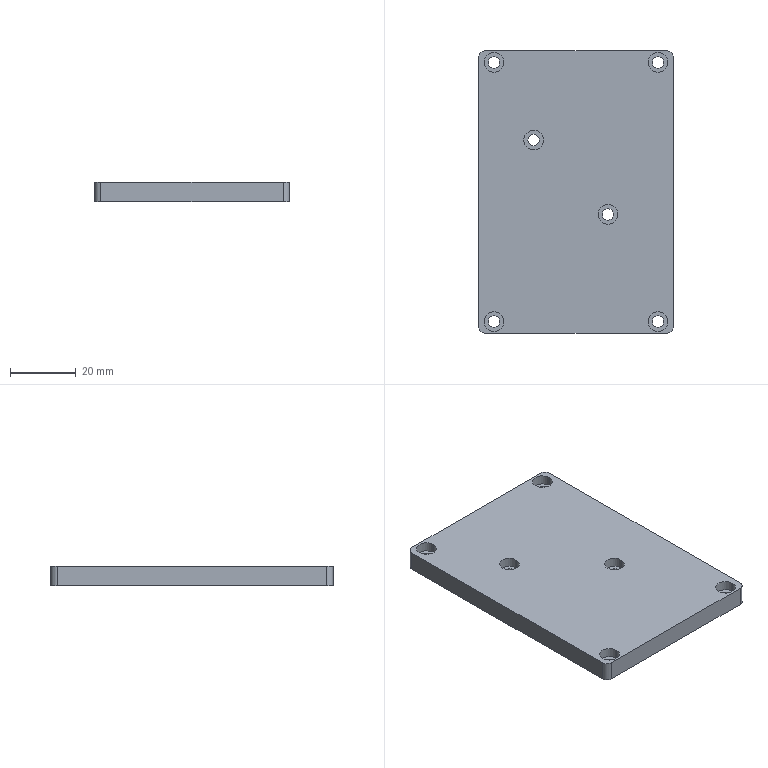Part | SolidWorks | features ICE 2, Extrusion 1, Fillet 1 | 1 solid | 40 faces | box 59.5 x 86 x 6 mm | volume 29999 mm3 | cylinder 28 | plane 12 | commonest cylinder face diameters 3.5 x12 6 x12 4 x4
STEP:
#1=CARTESIAN_POINT('',(22.,-39.5,3.));
#2=VERTEX_POINT('',#1);
#3=CARTESIAN_POINT('',(28.,-39.5,3.));
#4=VERTEX_POINT('',#3);
#5=CARTESIAN_POINT('',(25.,-39.5,3.));
#6=DIRECTION('',(0.,0.,1.));
#7=DIRECTION('',(1.,0.,0.));
#8=AXIS2_PLACEMENT_3D('',#5,#6,#7);
#9=CIRCLE('',#8,3.);
#10=EDGE_CURVE('',#2,#4,#9,.T.);
#11=ORIENTED_EDGE('',*,*,#10,.F.);
#12=CARTESIAN_POINT('',(22.,-39.5,6.));
#13=VERTEX_POINT('',#12);
#14=CARTESIAN_POINT('',(22.,-39.5,3.));
#15=DIRECTION('',(0.,0.,1.));
#16=VECTOR('',#15,1000.);
#17=LINE('',#14,#16);
#18=EDGE_CURVE('',#2,#13,#17,.T.);
#19=ORIENTED_EDGE('',*,*,#18,.T.);
#20=CARTESIAN_POINT('',(28.,-39.5,6.));
#21=VERTEX_POINT('',#20);
#22=CARTESIAN_POINT('',(25.,-39.5,6.));
#23=DIRECTION('',(0.,0.,1.));
#24=DIRECTION('',(1.,0.,0.));
#25=AXIS2_PLACEMENT_3D('',#22,#23,#24);
#26=CIRCLE('',#25,3.);
#27=EDGE_CURVE('',#13,#21,#26,.T.);
#28=ORIENTED_EDGE('',*,*,#27,.T.);
#29=CARTESIAN_POINT('',(28.,-39.5,3.));
#30=DIRECTION('',(0.,0.,1.));
#31=VECTOR('',#30,1000.);
#32=LINE('',#29,#31);
#33=EDGE_CURVE('',#4,#21,#32,.T.);
#34=ORIENTED_EDGE('',*,*,#33,.F.);
#35=EDGE_LOOP('',(#11,#19,#28,#34));
#36=FACE_OUTER_BOUND('',#35,.T.);
#37=CARTESIAN_POINT('',(25.,-39.5,3.));
#38=DIRECTION('',(0.,0.,1.));
#39=DIRECTION('',(1.,0.,0.));
#40=AXIS2_PLACEMENT_3D('',#37,#38,#39);
#41=CYLINDRICAL_SURFACE('',#40,3.);
#42=ADVANCED_FACE('',(#36),#41,.F.);
#43=CARTESIAN_POINT('',(-28.,-39.5,3.));
#44=VERTEX_POINT('',#43);
#45=CARTESIAN_POINT('',(-22.,-39.5,3.));
#46=VERTEX_POINT('',#45);
#47=CARTESIAN_POINT('',(-25.,-39.5,3.));
#48=DIRECTION('',(0.,0.,1.));
#49=DIRECTION('',(1.,0.,0.));
#50=AXIS2_PLACEMENT_3D('',#47,#48,#49);
#51=CIRCLE('',#50,3.);
#52=EDGE_CURVE('',#44,#46,#51,.T.);
#53=ORIENTED_EDGE('',*,*,#52,.F.);
#54=CARTESIAN_POINT('',(-28.,-39.5,6.));
#55=VERTEX_POINT('',#54);
#56=CARTESIAN_POINT('',(-28.,-39.5,3.));
#57=DIRECTION('',(0.,0.,1.));
#58=VECTOR('',#57,1000.);
#59=LINE('',#56,#58);
#60=EDGE_CURVE('',#44,#55,#59,.T.);
#61=ORIENTED_EDGE('',*,*,#60,.T.);
#62=CARTESIAN_POINT('',(-22.,-39.5,6.));
#63=VERTEX_POINT('',#62);
#64=CARTESIAN_POINT('',(-25.,-39.5,6.));
#65=DIRECTION('',(0.,0.,1.));
#66=DIRECTION('',(1.,0.,0.));
#67=AXIS2_PLACEMENT_3D('',#64,#65,#66);
#68=CIRCLE('',#67,3.);
#69=EDGE_CURVE('',#55,#63,#68,.T.);
#70=ORIENTED_EDGE('',*,*,#69,.T.);
#71=CARTESIAN_POINT('',(-22.,-39.5,3.));
#72=DIRECTION('',(0.,0.,1.));
#73=VECTOR('',#72,1000.);
#74=LINE('',#71,#73);
#75=EDGE_CURVE('',#46,#63,#74,.T.);
#76=ORIENTED_EDGE('',*,*,#75,.F.);
#77=EDGE_LOOP('',(#53,#61,#70,#76));
#78=FACE_OUTER_BOUND('',#77,.T.);
#79=CARTESIAN_POINT('',(-25.,-39.5,3.));
#80=DIRECTION('',(0.,0.,1.));
#81=DIRECTION('',(1.,0.,0.));
#82=AXIS2_PLACEMENT_3D('',#79,#80,#81);
#83=CYLINDRICAL_SURFACE('',#82,3.);
#84=ADVANCED_FACE('',(#78),#83,.F.);
#85=CARTESIAN_POINT('',(6.727,-6.827,3.));
#86=VERTEX_POINT('',#85);
#87=CARTESIAN_POINT('',(12.727,-6.827,3.));
#88=VERTEX_POINT('',#87);
#89=CARTESIAN_POINT('',(9.727,-6.827,3.));
#90=DIRECTION('',(0.,0.,1.));
#91=DIRECTION('',(1.,0.,0.));
#92=AXIS2_PLACEMENT_3D('',#89,#90,#91);
#93=CIRCLE('',#92,3.);
#94=EDGE_CURVE('',#86,#88,#93,.T.);
#95=ORIENTED_EDGE('',*,*,#94,.F.);
#96=CARTESIAN_POINT('',(6.727,-6.827,6.));
#97=VERTEX_POINT('',#96);
#98=CARTESIAN_POINT('',(6.727,-6.827,3.));
#99=DIRECTION('',(0.,0.,1.));
#100=VECTOR('',#99,1000.);
#101=LINE('',#98,#100);
#102=EDGE_CURVE('',#86,#97,#101,.T.);
#103=ORIENTED_EDGE('',*,*,#102,.T.);
#104=CARTESIAN_POINT('',(12.727,-6.827,6.));
#105=VERTEX_POINT('',#104);
#106=CARTESIAN_POINT('',(9.727,-6.827,6.));
#107=DIRECTION('',(0.,0.,1.));
#108=DIRECTION('',(1.,0.,0.));
#109=AXIS2_PLACEMENT_3D('',#106,#107,#108);
#110=CIRCLE('',#109,3.);
#111=EDGE_CURVE('',#97,#105,#110,.T.);
#112=ORIENTED_EDGE('',*,*,#111,.T.);
#113=CARTESIAN_POINT('',(12.727,-6.827,3.));
#114=DIRECTION('',(0.,0.,1.));
#115=VECTOR('',#114,1000.);
#116=LINE('',#113,#115);
#117=EDGE_CURVE('',#88,#105,#116,.T.);
#118=ORIENTED_EDGE('',*,*,#117,.F.);
#119=EDGE_LOOP('',(#95,#103,#112,#118));
#120=FACE_OUTER_BOUND('',#119,.T.);
#121=CARTESIAN_POINT('',(9.727,-6.827,3.));
#122=DIRECTION('',(0.,0.,1.));
#123=DIRECTION('',(1.,0.,0.));
#124=AXIS2_PLACEMENT_3D('',#121,#122,#123);
#125=CYLINDRICAL_SURFACE('',#124,3.);
#126=ADVANCED_FACE('',(#120),#125,.F.);
#127=CARTESIAN_POINT('',(-15.9,15.8,3.));
#128=VERTEX_POINT('',#127);
#129=CARTESIAN_POINT('',(-9.9,15.8,3.));
#130=VERTEX_POINT('',#129);
#131=CARTESIAN_POINT('',(-12.9,15.8,3.));
#132=DIRECTION('',(0.,0.,1.));
#133=DIRECTION('',(1.,0.,0.));
#134=AXIS2_PLACEMENT_3D('',#131,#132,#133);
#135=CIRCLE('',#134,3.);
#136=EDGE_CURVE('',#128,#130,#135,.T.);
#137=ORIENTED_EDGE('',*,*,#136,.F.);
#138=CARTESIAN_POINT('',(-15.9,15.8,6.));
#139=VERTEX_POINT('',#138);
#140=CARTESIAN_POINT('',(-15.9,15.8,3.));
#141=DIRECTION('',(0.,0.,1.));
#142=VECTOR('',#141,1000.);
#143=LINE('',#140,#142);
#144=EDGE_CURVE('',#128,#139,#143,.T.);
#145=ORIENTED_EDGE('',*,*,#144,.T.);
#146=CARTESIAN_POINT('',(-9.9,15.8,6.));
#147=VERTEX_POINT('',#146);
#148=CARTESIAN_POINT('',(-12.9,15.8,6.));
#149=DIRECTION('',(0.,0.,1.));
#150=DIRECTION('',(1.,0.,0.));
#151=AXIS2_PLACEMENT_3D('',#148,#149,#150);
#152=CIRCLE('',#151,3.);
#153=EDGE_CURVE('',#139,#147,#152,.T.);
#154=ORIENTED_EDGE('',*,*,#153,.T.);
#155=CARTESIAN_POINT('',(-9.9,15.8,3.));
#156=DIRECTION('',(0.,0.,1.));
#157=VECTOR('',#156,1000.);
#158=LINE('',#155,#157);
#159=EDGE_CURVE('',#130,#147,#158,.T.);
#160=ORIENTED_EDGE('',*,*,#159,.F.);
#161=EDGE_LOOP('',(#137,#145,#154,#160));
#162=FACE_OUTER_BOUND('',#161,.T.);
#163=CARTESIAN_POINT('',(-12.9,15.8,3.));
#164=DIRECTION('',(0.,0.,1.));
#165=DIRECTION('',(1.,0.,0.));
#166=AXIS2_PLACEMENT_3D('',#163,#164,#165);
#167=CYLINDRICAL_SURFACE('',#166,3.);
#168=ADVANCED_FACE('',(#162),#167,.F.);
#169=CARTESIAN_POINT('',(22.,39.5,3.));
#170=VERTEX_POINT('',#169);
#171=CARTESIAN_POINT('',(28.,39.5,3.));
#172=VERTEX_POINT('',#171);
#173=CARTESIAN_POINT('',(25.,39.5,3.));
#174=DIRECTION('',(0.,0.,1.));
#175=DIRECTION('',(1.,0.,0.));
#176=AXIS2_PLACEMENT_3D('',#173,#174,#175);
#177=CIRCLE('',#176,3.);
#178=EDGE_CURVE('',#170,#172,#177,.T.);
#179=ORIENTED_EDGE('',*,*,#178,.F.);
#180=CARTESIAN_POINT('',(22.,39.5,6.));
#181=VERTEX_POINT('',#180);
#182=CARTESIAN_POINT('',(22.,39.5,3.));
#183=DIRECTION('',(0.,0.,1.));
#184=VECTOR('',#183,1000.);
#185=LINE('',#182,#184);
#186=EDGE_CURVE('',#170,#181,#185,.T.);
#187=ORIENTED_EDGE('',*,*,#186,.T.);
#188=CARTESIAN_POINT('',(28.,39.5,6.));
#189=VERTEX_POINT('',#188);
#190=CARTESIAN_POINT('',(25.,39.5,6.));
#191=DIRECTION('',(0.,0.,1.));
#192=DIRECTION('',(1.,0.,0.));
#193=AXIS2_PLACEMENT_3D('',#190,#191,#192);
#194=CIRCLE('',#193,3.);
#195=EDGE_CURVE('',#181,#189,#194,.T.);
#196=ORIENTED_EDGE('',*,*,#195,.T.);
#197=CARTESIAN_POINT('',(28.,39.5,3.));
#198=DIRECTION('',(0.,0.,1.));
#199=VECTOR('',#198,1000.);
#200=LINE('',#197,#199);
#201=EDGE_CURVE('',#172,#189,#200,.T.);
#202=ORIENTED_EDGE('',*,*,#201,.F.);
#203=EDGE_LOOP('',(#179,#187,#196,#202));
#204=FACE_OUTER_BOUND('',#203,.T.);
#205=CARTESIAN_POINT('',(25.,39.5,3.));
#206=DIRECTION('',(0.,0.,1.));
#207=DIRECTION('',(1.,0.,0.));
#208=AXIS2_PLACEMENT_3D('',#205,#206,#207);
#209=CYLINDRICAL_SURFACE('',#208,3.);
#210=ADVANCED_FACE('',(#204),#209,.F.);
#211=CARTESIAN_POINT('',(-28.,39.5,3.));
#212=VERTEX_POINT('',#211);
#213=CARTESIAN_POINT('',(-22.,39.5,3.));
#214=VERTEX_POINT('',#213);
#215=CARTESIAN_POINT('',(-25.,39.5,3.));
#216=DIRECTION('',(0.,0.,1.));
#217=DIRECTION('',(1.,0.,0.));
#218=AXIS2_PLACEMENT_3D('',#215,#216,#217);
#219=CIRCLE('',#218,3.);
#220=EDGE_CURVE('',#212,#214,#219,.T.);
#221=ORIENTED_EDGE('',*,*,#220,.F.);
#222=CARTESIAN_POINT('',(-28.,39.5,6.));
#223=VERTEX_POINT('',#222);
#224=CARTESIAN_POINT('',(-28.,39.5,3.));
#225=DIRECTION('',(0.,0.,1.));
#226=VECTOR('',#225,1000.);
#227=LINE('',#224,#226);
#228=EDGE_CURVE('',#212,#223,#227,.T.);
#229=ORIENTED_EDGE('',*,*,#228,.T.);
#230=CARTESIAN_POINT('',(-22.,39.5,6.));
#231=VERTEX_POINT('',#230);
#232=CARTESIAN_POINT('',(-25.,39.5,6.));
#233=DIRECTION('',(0.,0.,1.));
#234=DIRECTION('',(1.,0.,0.));
#235=AXIS2_PLACEMENT_3D('',#232,#233,#234);
#236=CIRCLE('',#235,3.);
#237=EDGE_CURVE('',#223,#231,#236,.T.);
#238=ORIENTED_EDGE('',*,*,#237,.T.);
#239=CARTESIAN_POINT('',(-22.,39.5,3.));
#240=DIRECTION('',(0.,0.,1.));
#241=VECTOR('',#240,1000.);
#242=LINE('',#239,#241);
#243=EDGE_CURVE('',#214,#231,#242,.T.);
#244=ORIENTED_EDGE('',*,*,#243,.F.);
#245=EDGE_LOOP('',(#221,#229,#238,#244));
#246=FACE_OUTER_BOUND('',#245,.T.);
#247=CARTESIAN_POINT('',(-25.,39.5,3.));
#248=DIRECTION('',(0.,0.,1.));
#249=DIRECTION('',(1.,0.,0.));
#250=AXIS2_PLACEMENT_3D('',#247,#248,#249);
#251=CYLINDRICAL_SURFACE('',#250,3.);
#252=ADVANCED_FACE('',(#246),#251,.F.);
#253=CARTESIAN_POINT('',(-26.75,39.5,0.));
#254=VERTEX_POINT('',#253);
#255=CARTESIAN_POINT('',(-23.25,39.5,0.));
#256=VERTEX_POINT('',#255);
#257=CARTESIAN_POINT('',(-25.,39.5,0.));
#258=DIRECTION('',(0.,0.,1.));
#259=DIRECTION('',(1.,0.,0.));
#260=AXIS2_PLACEMENT_3D('',#257,#258,#259);
#261=CIRCLE('',#260,1.75);
#262=EDGE_CURVE('',#254,#256,#261,.T.);
#263=ORIENTED_EDGE('',*,*,#262,.F.);
#264=CARTESIAN_POINT('',(-26.75,39.5,3.));
#265=VERTEX_POINT('',#264);
#266=CARTESIAN_POINT('',(-26.75,39.5,0.));
#267=DIRECTION('',(0.,0.,1.));
#268=VECTOR('',#267,1000.);
#269=LINE('',#266,#268);
#270=EDGE_CURVE('',#254,#265,#269,.T.);
#271=ORIENTED_EDGE('',*,*,#270,.T.);
#272=CARTESIAN_POINT('',(-23.25,39.5,3.));
#273=VERTEX_POINT('',#272);
#274=CARTESIAN_POINT('',(-25.,39.5,3.));
#275=DIRECTION('',(0.,0.,-1.));
#276=DIRECTION('',(1.,0.,0.));
#277=AXIS2_PLACEMENT_3D('',#274,#275,#276);
#278=CIRCLE('',#277,1.75);
#279=EDGE_CURVE('',#273,#265,#278,.T.);
#280=ORIENTED_EDGE('',*,*,#279,.F.);
#281=CARTESIAN_POINT('',(-23.25,39.5,0.));
#282=DIRECTION('',(0.,0.,1.));
#283=VECTOR('',#282,1000.);
#284=LINE('',#281,#283);
#285=EDGE_CURVE('',#256,#273,#284,.T.);
#286=ORIENTED_EDGE('',*,*,#285,.F.);
#287=EDGE_LOOP('',(#263,#271,#280,#286));
#288=FACE_OUTER_BOUND('',#287,.T.);
#289=CARTESIAN_POINT('',(-25.,39.5,0.));
#290=DIRECTION('',(0.,0.,1.));
#291=DIRECTION('',(1.,0.,0.));
#292=AXIS2_PLACEMENT_3D('',#289,#290,#291);
#293=CYLINDRICAL_SURFACE('',#292,1.75);
#294=ADVANCED_FACE('',(#288),#293,.F.);
#295=CARTESIAN_POINT('',(23.25,39.5,0.));
#296=VERTEX_POINT('',#295);
#297=CARTESIAN_POINT('',(26.75,39.5,0.));
#298=VERTEX_POINT('',#297);
#299=CARTESIAN_POINT('',(25.,39.5,0.));
#300=DIRECTION('',(0.,0.,1.));
#301=DIRECTION('',(1.,0.,0.));
#302=AXIS2_PLACEMENT_3D('',#299,#300,#301);
#303=CIRCLE('',#302,1.75);
#304=EDGE_CURVE('',#296,#298,#303,.T.);
#305=ORIENTED_EDGE('',*,*,#304,.F.);
#306=CARTESIAN_POINT('',(23.25,39.5,3.));
#307=VERTEX_POINT('',#306);
#308=CARTESIAN_POINT('',(23.25,39.5,0.));
#309=DIRECTION('',(0.,0.,1.));
#310=VECTOR('',#309,1000.);
#311=LINE('',#308,#310);
#312=EDGE_CURVE('',#296,#307,#311,.T.);
#313=ORIENTED_EDGE('',*,*,#312,.T.);
#314=CARTESIAN_POINT('',(26.75,39.5,3.));
#315=VERTEX_POINT('',#314);
#316=CARTESIAN_POINT('',(25.,39.5,3.));
#317=DIRECTION('',(0.,0.,-1.));
#318=DIRECTION('',(1.,0.,0.));
#319=AXIS2_PLACEMENT_3D('',#316,#317,#318);
#320=CIRCLE('',#319,1.75);
#321=EDGE_CURVE('',#315,#307,#320,.T.);
#322=ORIENTED_EDGE('',*,*,#321,.F.);
#323=CARTESIAN_POINT('',(26.75,39.5,0.));
#324=DIRECTION('',(0.,0.,1.));
#325=VECTOR('',#324,1000.);
#326=LINE('',#323,#325);
#327=EDGE_CURVE('',#298,#315,#326,.T.);
#328=ORIENTED_EDGE('',*,*,#327,.F.);
#329=EDGE_LOOP('',(#305,#313,#322,#328));
#330=FACE_OUTER_BOUND('',#329,.T.);
#331=CARTESIAN_POINT('',(25.,39.5,0.));
#332=DIRECTION('',(0.,0.,1.));
#333=DIRECTION('',(1.,0.,0.));
#334=AXIS2_PLACEMENT_3D('',#331,#332,#333);
#335=CYLINDRICAL_SURFACE('',#334,1.75);
#336=ADVANCED_FACE('',(#330),#335,.F.);
#337=CARTESIAN_POINT('',(-14.65,15.8,0.));
#338=VERTEX_POINT('',#337);
#339=CARTESIAN_POINT('',(-11.15,15.8,0.));
#340=VERTEX_POINT('',#339);
#341=CARTESIAN_POINT('',(-12.9,15.8,0.));
#342=DIRECTION('',(0.,0.,1.));
#343=DIRECTION('',(1.,0.,0.));
#344=AXIS2_PLACEMENT_3D('',#341,#342,#343);
#345=CIRCLE('',#344,1.75);
#346=EDGE_CURVE('',#338,#340,#345,.T.);
#347=ORIENTED_EDGE('',*,*,#346,.F.);
#348=CARTESIAN_POINT('',(-14.65,15.8,3.));
#349=VERTEX_POINT('',#348);
#350=CARTESIAN_POINT('',(-14.65,15.8,0.));
#351=DIRECTION('',(0.,0.,1.));
#352=VECTOR('',#351,1000.);
#353=LINE('',#350,#352);
#354=EDGE_CURVE('',#338,#349,#353,.T.);
#355=ORIENTED_EDGE('',*,*,#354,.T.);
#356=CARTESIAN_POINT('',(-11.15,15.8,3.));
#357=VERTEX_POINT('',#356);
#358=CARTESIAN_POINT('',(-12.9,15.8,3.));
#359=DIRECTION('',(0.,0.,-1.));
#360=DIRECTION('',(1.,0.,0.));
#361=AXIS2_PLACEMENT_3D('',#358,#359,#360);
#362=CIRCLE('',#361,1.75);
#363=EDGE_CURVE('',#357,#349,#362,.T.);
#364=ORIENTED_EDGE('',*,*,#363,.F.);
#365=CARTESIAN_POINT('',(-11.15,15.8,0.));
#366=DIRECTION('',(0.,0.,1.));
#367=VECTOR('',#366,1000.);
#368=LINE('',#365,#367);
#369=EDGE_CURVE('',#340,#357,#368,.T.);
#370=ORIENTED_EDGE('',*,*,#369,.F.);
#371=EDGE_LOOP('',(#347,#355,#364,#370));
#372=FACE_OUTER_BOUND('',#371,.T.);
#373=CARTESIAN_POINT('',(-12.9,15.8,0.));
#374=DIRECTION('',(0.,0.,1.));
#375=DIRECTION('',(1.,0.,0.));
#376=AXIS2_PLACEMENT_3D('',#373,#374,#375);
#377=CYLINDRICAL_SURFACE('',#376,1.75);
#378=ADVANCED_FACE('',(#372),#377,.F.);
#379=CARTESIAN_POINT('',(7.977,-6.827,0.));
#380=VERTEX_POINT('',#379);
#381=CARTESIAN_POINT('',(11.477,-6.827,0.));
#382=VERTEX_POINT('',#381);
#383=CARTESIAN_POINT('',(9.727,-6.827,0.));
#384=DIRECTION('',(0.,0.,1.));
#385=DIRECTION('',(1.,0.,0.));
#386=AXIS2_PLACEMENT_3D('',#383,#384,#385);
#387=CIRCLE('',#386,1.75);
#388=EDGE_CURVE('',#380,#382,#387,.T.);
#389=ORIENTED_EDGE('',*,*,#388,.F.);
#390=CARTESIAN_POINT('',(7.977,-6.827,3.));
#391=VERTEX_POINT('',#390);
#392=CARTESIAN_POINT('',(7.977,-6.827,0.));
#393=DIRECTION('',(0.,0.,1.));
#394=VECTOR('',#393,1000.);
#395=LINE('',#392,#394);
#396=EDGE_CURVE('',#380,#391,#395,.T.);
#397=ORIENTED_EDGE('',*,*,#396,.T.);
#398=CARTESIAN_POINT('',(11.477,-6.827,3.));
#399=VERTEX_POINT('',#398);
#400=CARTESIAN_POINT('',(9.727,-6.827,3.));
#401=DIRECTION('',(0.,0.,-1.));
#402=DIRECTION('',(1.,0.,0.));
#403=AXIS2_PLACEMENT_3D('',#400,#401,#402);
#404=CIRCLE('',#403,1.75);
#405=EDGE_CURVE('',#399,#391,#404,.T.);
#406=ORIENTED_EDGE('',*,*,#405,.F.);
#407=CARTESIAN_POINT('',(11.477,-6.827,0.));
#408=DIRECTION('',(0.,0.,1.));
#409=VECTOR('',#408,1000.);
#410=LINE('',#407,#409);
#411=EDGE_CURVE('',#382,#399,#410,.T.);
#412=ORIENTED_EDGE('',*,*,#411,.F.);
#413=EDGE_LOOP('',(#389,#397,#406,#412));
#414=FACE_OUTER_BOUND('',#413,.T.);
#415=CARTESIAN_POINT('',(9.727,-6.827,0.));
#416=DIRECTION('',(0.,0.,1.));
#417=DIRECTION('',(1.,0.,0.));
#418=AXIS2_PLACEMENT_3D('',#415,#416,#417);
#419=CYLINDRICAL_SURFACE('',#418,1.75);
#420=ADVANCED_FACE('',(#414),#419,.F.);
#421=CARTESIAN_POINT('',(-26.75,-39.5,0.));
#422=VERTEX_POINT('',#421);
#423=CARTESIAN_POINT('',(-23.25,-39.5,0.));
#424=VERTEX_POINT('',#423);
#425=CARTESIAN_POINT('',(-25.,-39.5,0.));
#426=DIRECTION('',(0.,0.,1.));
#427=DIRECTION('',(1.,0.,0.));
#428=AXIS2_PLACEMENT_3D('',#425,#426,#427);
#429=CIRCLE('',#428,1.75);
#430=EDGE_CURVE('',#422,#424,#429,.T.);
#431=ORIENTED_EDGE('',*,*,#430,.F.);
#432=CARTESIAN_POINT('',(-26.75,-39.5,3.));
#433=VERTEX_POINT('',#432);
#434=CARTESIAN_POINT('',(-26.75,-39.5,0.));
#435=DIRECTION('',(0.,0.,1.));
#436=VECTOR('',#435,1000.);
#437=LINE('',#434,#436);
#438=EDGE_CURVE('',#422,#433,#437,.T.);
#439=ORIENTED_EDGE('',*,*,#438,.T.);
#440=CARTESIAN_POINT('',(-23.25,-39.5,3.));
#441=VERTEX_POINT('',#440);
#442=CARTESIAN_POINT('',(-25.,-39.5,3.));
#443=DIRECTION('',(0.,0.,-1.));
#444=DIRECTION('',(1.,0.,0.));
#445=AXIS2_PLACEMENT_3D('',#442,#443,#444);
#446=CIRCLE('',#445,1.75);
#447=EDGE_CURVE('',#441,#433,#446,.T.);
#448=ORIENTED_EDGE('',*,*,#447,.F.);
#449=CARTESIAN_POINT('',(-23.25,-39.5,0.));
#450=DIRECTION('',(0.,0.,1.));
#451=VECTOR('',#450,1000.);
#452=LINE('',#449,#451);
#453=EDGE_CURVE('',#424,#441,#452,.T.);
#454=ORIENTED_EDGE('',*,*,#453,.F.);
#455=EDGE_LOOP('',(#431,#439,#448,#454));
#456=FACE_OUTER_BOUND('',#455,.T.);
#457=CARTESIAN_POINT('',(-25.,-39.5,0.));
#458=DIRECTION('',(0.,0.,1.));
#459=DIRECTION('',(1.,0.,0.));
#460=AXIS2_PLACEMENT_3D('',#457,#458,#459);
#461=CYLINDRICAL_SURFACE('',#460,1.75);
#462=ADVANCED_FACE('',(#456),#461,.F.);
#463=CARTESIAN_POINT('',(23.25,-39.5,0.));
#464=VERTEX_POINT('',#463);
#465=CARTESIAN_POINT('',(26.75,-39.5,0.));
#466=VERTEX_POINT('',#465);
#467=CARTESIAN_POINT('',(25.,-39.5,0.));
#468=DIRECTION('',(0.,0.,1.));
#469=DIRECTION('',(1.,0.,0.));
#470=AXIS2_PLACEMENT_3D('',#467,#468,#469);
#471=CIRCLE('',#470,1.75);
#472=EDGE_CURVE('',#464,#466,#471,.T.);
#473=ORIENTED_EDGE('',*,*,#472,.F.);
#474=CARTESIAN_POINT('',(23.25,-39.5,3.));
#475=VERTEX_POINT('',#474);
#476=CARTESIAN_POINT('',(23.25,-39.5,0.));
#477=DIRECTION('',(0.,0.,1.));
#478=VECTOR('',#477,1000.);
#479=LINE('',#476,#478);
#480=EDGE_CURVE('',#464,#475,#479,.T.);
#481=ORIENTED_EDGE('',*,*,#480,.T.);
#482=CARTESIAN_POINT('',(26.75,-39.5,3.));
#483=VERTEX_POINT('',#482);
#484=CARTESIAN_POINT('',(25.,-39.5,3.));
#485=DIRECTION('',(0.,0.,-1.));
#486=DIRECTION('',(1.,0.,0.));
#487=AXIS2_PLACEMENT_3D('',#484,#485,#486);
#488=CIRCLE('',#487,1.75);
#489=EDGE_CURVE('',#483,#475,#488,.T.);
#490=ORIENTED_EDGE('',*,*,#489,.F.);
#491=CARTESIAN_POINT('',(26.75,-39.5,0.));
#492=DIRECTION('',(0.,0.,1.));
#493=VECTOR('',#492,1000.);
#494=LINE('',#491,#493);
#495=EDGE_CURVE('',#466,#483,#494,.T.);
#496=ORIENTED_EDGE('',*,*,#495,.F.);
#497=EDGE_LOOP('',(#473,#481,#490,#496));
#498=FACE_OUTER_BOUND('',#497,.T.);
#499=CARTESIAN_POINT('',(25.,-39.5,0.));
#500=DIRECTION('',(0.,0.,1.));
#501=DIRECTION('',(1.,0.,0.));
#502=AXIS2_PLACEMENT_3D('',#499,#500,#501);
#503=CYLINDRICAL_SURFACE('',#502,1.75);
#504=ADVANCED_FACE('',(#498),#503,.F.);
#505=ORIENTED_EDGE('',*,*,#480,.F.);
#506=CARTESIAN_POINT('',(25.,-39.5,0.));
#507=DIRECTION('',(0.,0.,1.));
#508=DIRECTION('',(1.,0.,0.));
#509=AXIS2_PLACEMENT_3D('',#506,#507,#508);
#510=CIRCLE('',#509,1.75);
#511=EDGE_CURVE('',#466,#464,#510,.T.);
#512=ORIENTED_EDGE('',*,*,#511,.F.);
#513=ORIENTED_EDGE('',*,*,#495,.T.);
#514=CARTESIAN_POINT('',(25.,-39.5,3.));
#515=DIRECTION('',(0.,0.,-1.));
#516=DIRECTION('',(1.,0.,0.));
#517=AXIS2_PLACEMENT_3D('',#514,#515,#516);
#518=CIRCLE('',#517,1.75);
#519=EDGE_CURVE('',#475,#483,#518,.T.);
#520=ORIENTED_EDGE('',*,*,#519,.F.);
#521=EDGE_LOOP('',(#505,#512,#513,#520));
#522=FACE_OUTER_BOUND('',#521,.T.);
#523=CARTESIAN_POINT('',(25.,-39.5,0.));
#524=DIRECTION('',(0.,0.,1.));
#525=DIRECTION('',(1.,0.,0.));
#526=AXIS2_PLACEMENT_3D('',#523,#524,#525);
#527=CYLINDRICAL_SURFACE('',#526,1.75);
#528=ADVANCED_FACE('',(#522),#527,.F.);
#529=ORIENTED_EDGE('',*,*,#438,.F.);
#530=CARTESIAN_POINT('',(-25.,-39.5,0.));
#531=DIRECTION('',(0.,0.,1.));
#532=DIRECTION('',(1.,0.,0.));
#533=AXIS2_PLACEMENT_3D('',#530,#531,#532);
#534=CIRCLE('',#533,1.75);
#535=EDGE_CURVE('',#424,#422,#534,.T.);
#536=ORIENTED_EDGE('',*,*,#535,.F.);
#537=ORIENTED_EDGE('',*,*,#453,.T.);
#538=CARTESIAN_POINT('',(-25.,-39.5,3.));
#539=DIRECTION('',(0.,0.,-1.));
#540=DIRECTION('',(1.,0.,0.));
#541=AXIS2_PLACEMENT_3D('',#538,#539,#540);
#542=CIRCLE('',#541,1.75);
#543=EDGE_CURVE('',#433,#441,#542,.T.);
#544=ORIENTED_EDGE('',*,*,#543,.F.);
#545=EDGE_LOOP('',(#529,#536,#537,#544));
#546=FACE_OUTER_BOUND('',#545,.T.);
#547=CARTESIAN_POINT('',(-25.,-39.5,0.));
#548=DIRECTION('',(0.,0.,1.));
#549=DIRECTION('',(1.,0.,0.));
#550=AXIS2_PLACEMENT_3D('',#547,#548,#549);
#551=CYLINDRICAL_SURFACE('',#550,1.75);
#552=ADVANCED_FACE('',(#546),#551,.F.);
#553=ORIENTED_EDGE('',*,*,#396,.F.);
#554=CARTESIAN_POINT('',(9.727,-6.827,0.));
#555=DIRECTION('',(0.,0.,1.));
#556=DIRECTION('',(1.,0.,0.));
#557=AXIS2_PLACEMENT_3D('',#554,#555,#556);
#558=CIRCLE('',#557,1.75);
#559=EDGE_CURVE('',#382,#380,#558,.T.);
#560=ORIENTED_EDGE('',*,*,#559,.F.);
#561=ORIENTED_EDGE('',*,*,#411,.T.);
#562=CARTESIAN_POINT('',(9.727,-6.827,3.));
#563=DIRECTION('',(0.,0.,-1.));
#564=DIRECTION('',(1.,0.,0.));
#565=AXIS2_PLACEMENT_3D('',#562,#563,#564);
#566=CIRCLE('',#565,1.75);
#567=EDGE_CURVE('',#391,#399,#566,.T.);
#568=ORIENTED_EDGE('',*,*,#567,.F.);
#569=EDGE_LOOP('',(#553,#560,#561,#568));
#570=FACE_OUTER_BOUND('',#569,.T.);
#571=CARTESIAN_POINT('',(9.727,-6.827,0.));
#572=DIRECTION('',(0.,0.,1.));
#573=DIRECTION('',(1.,0.,0.));
#574=AXIS2_PLACEMENT_3D('',#571,#572,#573);
#575=CYLINDRICAL_SURFACE('',#574,1.75);
#576=ADVANCED_FACE('',(#570),#575,.F.);
#577=ORIENTED_EDGE('',*,*,#354,.F.);
#578=CARTESIAN_POINT('',(-12.9,15.8,0.));
#579=DIRECTION('',(0.,0.,1.));
#580=DIRECTION('',(1.,0.,0.));
#581=AXIS2_PLACEMENT_3D('',#578,#579,#580);
#582=CIRCLE('',#581,1.75);
#583=EDGE_CURVE('',#340,#338,#582,.T.);
#584=ORIENTED_EDGE('',*,*,#583,.F.);
#585=ORIENTED_EDGE('',*,*,#369,.T.);
#586=CARTESIAN_POINT('',(-12.9,15.8,3.));
#587=DIRECTION('',(0.,0.,-1.));
#588=DIRECTION('',(1.,0.,0.));
#589=AXIS2_PLACEMENT_3D('',#586,#587,#588);
#590=CIRCLE('',#589,1.75);
#591=EDGE_CURVE('',#349,#357,#590,.T.);
#592=ORIENTED_EDGE('',*,*,#591,.F.);
#593=EDGE_LOOP('',(#577,#584,#585,#592));
#594=FACE_OUTER_BOUND('',#593,.T.);
#595=CARTESIAN_POINT('',(-12.9,15.8,0.));
#596=DIRECTION('',(0.,0.,1.));
#597=DIRECTION('',(1.,0.,0.));
#598=AXIS2_PLACEMENT_3D('',#595,#596,#597);
#599=CYLINDRICAL_SURFACE('',#598,1.75);
#600=ADVANCED_FACE('',(#594),#599,.F.);
#601=ORIENTED_EDGE('',*,*,#312,.F.);
#602=CARTESIAN_POINT('',(25.,39.5,0.));
#603=DIRECTION('',(0.,0.,1.));
#604=DIRECTION('',(1.,0.,0.));
#605=AXIS2_PLACEMENT_3D('',#602,#603,#604);
#606=CIRCLE('',#605,1.75);
#607=EDGE_CURVE('',#298,#296,#606,.T.);
#608=ORIENTED_EDGE('',*,*,#607,.F.);
#609=ORIENTED_EDGE('',*,*,#327,.T.);
#610=CARTESIAN_POINT('',(25.,39.5,3.));
#611=DIRECTION('',(0.,0.,-1.));
#612=DIRECTION('',(1.,0.,0.));
#613=AXIS2_PLACEMENT_3D('',#610,#611,#612);
#614=CIRCLE('',#613,1.75);
#615=EDGE_CURVE('',#307,#315,#614,.T.);
#616=ORIENTED_EDGE('',*,*,#615,.F.);
#617=EDGE_LOOP('',(#601,#608,#609,#616));
#618=FACE_OUTER_BOUND('',#617,.T.);
#619=CARTESIAN_POINT('',(25.,39.5,0.));
#620=DIRECTION('',(0.,0.,1.));
#621=DIRECTION('',(1.,0.,0.));
#622=AXIS2_PLACEMENT_3D('',#619,#620,#621);
#623=CYLINDRICAL_SURFACE('',#622,1.75);
#624=ADVANCED_FACE('',(#618),#623,.F.);
#625=ORIENTED_EDGE('',*,*,#270,.F.);
#626=CARTESIAN_POINT('',(-25.,39.5,0.));
#627=DIRECTION('',(0.,0.,1.));
#628=DIRECTION('',(1.,0.,0.));
#629=AXIS2_PLACEMENT_3D('',#626,#627,#628);
#630=CIRCLE('',#629,1.75);
#631=EDGE_CURVE('',#256,#254,#630,.T.);
#632=ORIENTED_EDGE('',*,*,#631,.F.);
#633=ORIENTED_EDGE('',*,*,#285,.T.);
#634=CARTESIAN_POINT('',(-25.,39.5,3.));
#635=DIRECTION('',(0.,0.,-1.));
#636=DIRECTION('',(1.,0.,0.));
#637=AXIS2_PLACEMENT_3D('',#634,#635,#636);
#638=CIRCLE('',#637,1.75);
#639=EDGE_CURVE('',#265,#273,#638,.T.);
#640=ORIENTED_EDGE('',*,*,#639,.F.);
#641=EDGE_LOOP('',(#625,#632,#633,#640));
#642=FACE_OUTER_BOUND('',#641,.T.);
#643=CARTESIAN_POINT('',(-25.,39.5,0.));
#644=DIRECTION('',(0.,0.,1.));
#645=DIRECTION('',(1.,0.,0.));
#646=AXIS2_PLACEMENT_3D('',#643,#644,#645);
#647=CYLINDRICAL_SURFACE('',#646,1.75);
#648=ADVANCED_FACE('',(#642),#647,.F.);
#649=CARTESIAN_POINT('',(29.75,-41.,6.));
#650=VERTEX_POINT('',#649);
#651=CARTESIAN_POINT('',(29.75,41.,6.));
#652=VERTEX_POINT('',#651);
#653=CARTESIAN_POINT('',(29.75,43.,6.));
#654=DIRECTION('',(0.,1.,0.));
#655=VECTOR('',#654,1000.);
#656=LINE('',#653,#655);
#657=EDGE_CURVE('',#650,#652,#656,.T.);
#658=ORIENTED_EDGE('',*,*,#657,.F.);
#659=CARTESIAN_POINT('',(29.75,-41.,0.));
#660=VERTEX_POINT('',#659);
#661=CARTESIAN_POINT('',(29.75,-41.,6.));
#662=DIRECTION('',(0.,0.,-1.));
#663=VECTOR('',#662,1000.);
#664=LINE('',#661,#663);
#665=EDGE_CURVE('',#650,#660,#664,.T.);
#666=ORIENTED_EDGE('',*,*,#665,.T.);
#667=CARTESIAN_POINT('',(29.75,41.,0.));
#668=VERTEX_POINT('',#667);
#669=CARTESIAN_POINT('',(29.75,43.,0.));
#670=DIRECTION('',(0.,1.,0.));
#671=VECTOR('',#670,1000.);
#672=LINE('',#669,#671);
#673=EDGE_CURVE('',#660,#668,#672,.T.);
#674=ORIENTED_EDGE('',*,*,#673,.T.);
#675=CARTESIAN_POINT('',(29.75,41.,6.));
#676=DIRECTION('',(0.,0.,1.));
#677=VECTOR('',#676,1000.);
#678=LINE('',#675,#677);
#679=EDGE_CURVE('',#668,#652,#678,.T.);
#680=ORIENTED_EDGE('',*,*,#679,.T.);
#681=EDGE_LOOP('',(#658,#666,#674,#680));
#682=FACE_OUTER_BOUND('',#681,.T.);
#683=CARTESIAN_POINT('',(29.75,43.,6.));
#684=DIRECTION('',(-1.,0.,0.));
#685=DIRECTION('',(0.,0.,1.));
#686=AXIS2_PLACEMENT_3D('',#683,#684,#685);
#687=PLANE('',#686);
#688=ADVANCED_FACE('',(#682),#687,.F.);
#689=CARTESIAN_POINT('',(27.75,43.,6.));
#690=VERTEX_POINT('',#689);
#691=CARTESIAN_POINT('',(-27.75,43.,6.));
#692=VERTEX_POINT('',#691);
#693=CARTESIAN_POINT('',(-29.75,43.,6.));
#694=DIRECTION('',(-1.,0.,0.));
#695=VECTOR('',#694,1000.);
#696=LINE('',#693,#695);
#697=EDGE_CURVE('',#690,#692,#696,.T.);
#698=ORIENTED_EDGE('',*,*,#697,.F.);
#699=CARTESIAN_POINT('',(27.75,43.,0.));
#700=VERTEX_POINT('',#699);
#701=CARTESIAN_POINT('',(27.75,43.,6.));
#702=DIRECTION('',(0.,0.,-1.));
#703=VECTOR('',#702,1000.);
#704=LINE('',#701,#703);
#705=EDGE_CURVE('',#690,#700,#704,.T.);
#706=ORIENTED_EDGE('',*,*,#705,.T.);
#707=CARTESIAN_POINT('',(-27.75,43.,0.));
#708=VERTEX_POINT('',#707);
#709=CARTESIAN_POINT('',(-29.75,43.,0.));
#710=DIRECTION('',(-1.,0.,0.));
#711=VECTOR('',#710,1000.);
#712=LINE('',#709,#711);
#713=EDGE_CURVE('',#700,#708,#712,.T.);
#714=ORIENTED_EDGE('',*,*,#713,.T.);
#715=CARTESIAN_POINT('',(-27.75,43.,6.));
#716=DIRECTION('',(0.,0.,1.));
#717=VECTOR('',#716,1000.);
#718=LINE('',#715,#717);
#719=EDGE_CURVE('',#708,#692,#718,.T.);
#720=ORIENTED_EDGE('',*,*,#719,.T.);
#721=EDGE_LOOP('',(#698,#706,#714,#720));
#722=FACE_OUTER_BOUND('',#721,.T.);
#723=CARTESIAN_POINT('',(-29.75,43.,6.));
#724=DIRECTION('',(0.,-1.,0.));
#725=DIRECTION('',(0.,0.,-1.));
#726=AXIS2_PLACEMENT_3D('',#723,#724,#725);
#727=PLANE('',#726);
#728=ADVANCED_FACE('',(#722),#727,.F.);
#729=CARTESIAN_POINT('',(-29.75,41.,0.));
#730=VERTEX_POINT('',#729);
#731=CARTESIAN_POINT('',(-29.75,-41.,0.));
#732=VERTEX_POINT('',#731);
#733=CARTESIAN_POINT('',(-29.75,43.,0.));
#734=DIRECTION('',(0.,-1.,0.));
#735=VECTOR('',#734,1000.);
#736=LINE('',#733,#735);
#737=EDGE_CURVE('',#730,#732,#736,.T.);
#738=ORIENTED_EDGE('',*,*,#737,.T.);
#739=CARTESIAN_POINT('',(-29.75,-41.,6.));
#740=VERTEX_POINT('',#739);
#741=CARTESIAN_POINT('',(-29.75,-41.,6.));
#742=DIRECTION('',(0.,0.,1.));
#743=VECTOR('',#742,1000.);
#744=LINE('',#741,#743);
#745=EDGE_CURVE('',#732,#740,#744,.T.);
#746=ORIENTED_EDGE('',*,*,#745,.T.);
#747=CARTESIAN_POINT('',(-29.75,41.,6.));
#748=VERTEX_POINT('',#747);
#749=CARTESIAN_POINT('',(-29.75,43.,6.));
#750=DIRECTION('',(0.,-1.,0.));
#751=VECTOR('',#750,1000.);
#752=LINE('',#749,#751);
#753=EDGE_CURVE('',#748,#740,#752,.T.);
#754=ORIENTED_EDGE('',*,*,#753,.F.);
#755=CARTESIAN_POINT('',(-29.75,41.,6.));
#756=DIRECTION('',(0.,0.,-1.));
#757=VECTOR('',#756,1000.);
#758=LINE('',#755,#757);
#759=EDGE_CURVE('',#748,#730,#758,.T.);
#760=ORIENTED_EDGE('',*,*,#759,.T.);
#761=EDGE_LOOP('',(#738,#746,#754,#760));
#762=FACE_OUTER_BOUND('',#761,.T.);
#763=CARTESIAN_POINT('',(-29.75,43.,6.));
#764=DIRECTION('',(1.,0.,0.));
#765=DIRECTION('',(0.,0.,-1.));
#766=AXIS2_PLACEMENT_3D('',#763,#764,#765);
#767=PLANE('',#766);
#768=ADVANCED_FACE('',(#762),#767,.F.);
#769=CARTESIAN_POINT('',(-27.75,-43.,6.));
#770=VERTEX_POINT('',#769);
#771=CARTESIAN_POINT('',(27.75,-43.,6.));
#772=VERTEX_POINT('',#771);
#773=CARTESIAN_POINT('',(-29.75,-43.,6.));
#774=DIRECTION('',(1.,0.,0.));
#775=VECTOR('',#774,1000.);
#776=LINE('',#773,#775);
#777=EDGE_CURVE('',#770,#772,#776,.T.);
#778=ORIENTED_EDGE('',*,*,#777,.F.);
#779=CARTESIAN_POINT('',(-27.75,-43.,0.));
#780=VERTEX_POINT('',#779);
#781=CARTESIAN_POINT('',(-27.75,-43.,6.));
#782=DIRECTION('',(0.,0.,-1.));
#783=VECTOR('',#782,1000.);
#784=LINE('',#781,#783);
#785=EDGE_CURVE('',#770,#780,#784,.T.);
#786=ORIENTED_EDGE('',*,*,#785,.T.);
#787=CARTESIAN_POINT('',(27.75,-43.,0.));
#788=VERTEX_POINT('',#787);
#789=CARTESIAN_POINT('',(-29.75,-43.,0.));
#790=DIRECTION('',(1.,0.,0.));
#791=VECTOR('',#790,1000.);
#792=LINE('',#789,#791);
#793=EDGE_CURVE('',#780,#788,#792,.T.);
#794=ORIENTED_EDGE('',*,*,#793,.T.);
#795=CARTESIAN_POINT('',(27.75,-43.,6.));
#796=DIRECTION('',(0.,0.,1.));
#797=VECTOR('',#796,1000.);
#798=LINE('',#795,#797);
#799=EDGE_CURVE('',#788,#772,#798,.T.);
#800=ORIENTED_EDGE('',*,*,#799,.T.);
#801=EDGE_LOOP('',(#778,#786,#794,#800));
#802=FACE_OUTER_BOUND('',#801,.T.);
#803=CARTESIAN_POINT('',(-29.75,-43.,6.));
#804=DIRECTION('',(0.,1.,0.));
#805=DIRECTION('',(0.,0.,1.));
#806=AXIS2_PLACEMENT_3D('',#803,#804,#805);
#807=PLANE('',#806);
#808=ADVANCED_FACE('',(#802),#807,.F.);
#809=CARTESIAN_POINT('',(25.,-39.5,6.));
#810=DIRECTION('',(0.,0.,1.));
#811=DIRECTION('',(1.,0.,0.));
#812=AXIS2_PLACEMENT_3D('',#809,#810,#811);
#813=CIRCLE('',#812,3.);
#814=EDGE_CURVE('',#21,#13,#813,.T.);
#815=ORIENTED_EDGE('',*,*,#814,.F.);
#816=ORIENTED_EDGE('',*,*,#27,.F.);
#817=EDGE_LOOP('',(#815,#816));
#818=FACE_BOUND('',#817,.T.);
#819=CARTESIAN_POINT('',(-25.,-39.5,6.));
#820=DIRECTION('',(0.,0.,1.));
#821=DIRECTION('',(1.,0.,0.));
#822=AXIS2_PLACEMENT_3D('',#819,#820,#821);
#823=CIRCLE('',#822,3.);
#824=EDGE_CURVE('',#63,#55,#823,.T.);
#825=ORIENTED_EDGE('',*,*,#824,.F.);
#826=ORIENTED_EDGE('',*,*,#69,.F.);
#827=EDGE_LOOP('',(#825,#826));
#828=FACE_BOUND('',#827,.T.);
#829=CARTESIAN_POINT('',(9.727,-6.827,6.));
#830=DIRECTION('',(0.,0.,1.));
#831=DIRECTION('',(1.,0.,0.));
#832=AXIS2_PLACEMENT_3D('',#829,#830,#831);
#833=CIRCLE('',#832,3.);
#834=EDGE_CURVE('',#105,#97,#833,.T.);
#835=ORIENTED_EDGE('',*,*,#834,.F.);
#836=ORIENTED_EDGE('',*,*,#111,.F.);
#837=EDGE_LOOP('',(#835,#836));
#838=FACE_BOUND('',#837,.T.);
#839=CARTESIAN_POINT('',(-12.9,15.8,6.));
#840=DIRECTION('',(0.,0.,1.));
#841=DIRECTION('',(1.,0.,0.));
#842=AXIS2_PLACEMENT_3D('',#839,#840,#841);
#843=CIRCLE('',#842,3.);
#844=EDGE_CURVE('',#147,#139,#843,.T.);
#845=ORIENTED_EDGE('',*,*,#844,.F.);
#846=ORIENTED_EDGE('',*,*,#153,.F.);
#847=EDGE_LOOP('',(#845,#846));
#848=FACE_BOUND('',#847,.T.);
#849=CARTESIAN_POINT('',(25.,39.5,6.));
#850=DIRECTION('',(0.,0.,1.));
#851=DIRECTION('',(1.,0.,0.));
#852=AXIS2_PLACEMENT_3D('',#849,#850,#851);
#853=CIRCLE('',#852,3.);
#854=EDGE_CURVE('',#189,#181,#853,.T.);
#855=ORIENTED_EDGE('',*,*,#854,.F.);
#856=ORIENTED_EDGE('',*,*,#195,.F.);
#857=EDGE_LOOP('',(#855,#856));
#858=FACE_BOUND('',#857,.T.);
#859=CARTESIAN_POINT('',(-25.,39.5,6.));
#860=DIRECTION('',(0.,0.,1.));
#861=DIRECTION('',(1.,0.,0.));
#862=AXIS2_PLACEMENT_3D('',#859,#860,#861);
#863=CIRCLE('',#862,3.);
#864=EDGE_CURVE('',#231,#223,#863,.T.);
#865=ORIENTED_EDGE('',*,*,#864,.F.);
#866=ORIENTED_EDGE('',*,*,#237,.F.);
#867=EDGE_LOOP('',(#865,#866));
#868=FACE_BOUND('',#867,.T.);
#869=ORIENTED_EDGE('',*,*,#753,.T.);
#870=CARTESIAN_POINT('',(-27.75,-41.,6.));
#871=DIRECTION('',(0.,0.,1.));
#872=DIRECTION('',(1.,0.,0.));
#873=AXIS2_PLACEMENT_3D('',#870,#871,#872);
#874=CIRCLE('',#873,2.);
#875=EDGE_CURVE('',#740,#770,#874,.T.);
#876=ORIENTED_EDGE('',*,*,#875,.T.);
#877=ORIENTED_EDGE('',*,*,#777,.T.);
#878=CARTESIAN_POINT('',(27.75,-41.,6.));
#879=DIRECTION('',(0.,0.,1.));
#880=DIRECTION('',(1.,0.,0.));
#881=AXIS2_PLACEMENT_3D('',#878,#879,#880);
#882=CIRCLE('',#881,2.);
#883=EDGE_CURVE('',#772,#650,#882,.T.);
#884=ORIENTED_EDGE('',*,*,#883,.T.);
#885=ORIENTED_EDGE('',*,*,#657,.T.);
#886=CARTESIAN_POINT('',(27.75,41.,6.));
#887=DIRECTION('',(0.,0.,1.));
#888=DIRECTION('',(1.,0.,0.));
#889=AXIS2_PLACEMENT_3D('',#886,#887,#888);
#890=CIRCLE('',#889,2.);
#891=EDGE_CURVE('',#652,#690,#890,.T.);
#892=ORIENTED_EDGE('',*,*,#891,.T.);
#893=ORIENTED_EDGE('',*,*,#697,.T.);
#894=CARTESIAN_POINT('',(-27.75,41.,6.));
#895=DIRECTION('',(0.,0.,1.));
#896=DIRECTION('',(1.,0.,0.));
#897=AXIS2_PLACEMENT_3D('',#894,#895,#896);
#898=CIRCLE('',#897,2.);
#899=EDGE_CURVE('',#692,#748,#898,.T.);
#900=ORIENTED_EDGE('',*,*,#899,.T.);
#901=EDGE_LOOP('',(#869,#876,#877,#884,#885,#892,#893,#900));
#902=FACE_OUTER_BOUND('',#901,.T.);
#903=CARTESIAN_POINT('',(29.75,-43.,6.));
#904=DIRECTION('',(0.,0.,1.));
#905=DIRECTION('',(1.,0.,0.));
#906=AXIS2_PLACEMENT_3D('',#903,#904,#905);
#907=PLANE('',#906);
#908=ADVANCED_FACE('',(#818,#828,#838,#848,#858,#868,#902),#907,.T.);
#909=ORIENTED_EDGE('',*,*,#559,.T.);
#910=ORIENTED_EDGE('',*,*,#388,.T.);
#911=EDGE_LOOP('',(#909,#910));
#912=FACE_BOUND('',#911,.T.);
#913=ORIENTED_EDGE('',*,*,#583,.T.);
#914=ORIENTED_EDGE('',*,*,#346,.T.);
#915=EDGE_LOOP('',(#913,#914));
#916=FACE_BOUND('',#915,.T.);
#917=ORIENTED_EDGE('',*,*,#631,.T.);
#918=ORIENTED_EDGE('',*,*,#262,.T.);
#919=EDGE_LOOP('',(#917,#918));
#920=FACE_BOUND('',#919,.T.);
#921=ORIENTED_EDGE('',*,*,#607,.T.);
#922=ORIENTED_EDGE('',*,*,#304,.T.);
#923=EDGE_LOOP('',(#921,#922));
#924=FACE_BOUND('',#923,.T.);
#925=ORIENTED_EDGE('',*,*,#511,.T.);
#926=ORIENTED_EDGE('',*,*,#472,.T.);
#927=EDGE_LOOP('',(#925,#926));
#928=FACE_BOUND('',#927,.T.);
#929=ORIENTED_EDGE('',*,*,#535,.T.);
#930=ORIENTED_EDGE('',*,*,#430,.T.);
#931=EDGE_LOOP('',(#929,#930));
#932=FACE_BOUND('',#931,.T.);
#933=ORIENTED_EDGE('',*,*,#793,.F.);
#934=CARTESIAN_POINT('',(-27.75,-41.,0.));
#935=DIRECTION('',(0.,0.,-1.));
#936=DIRECTION('',(1.,0.,0.));
#937=AXIS2_PLACEMENT_3D('',#934,#935,#936);
#938=CIRCLE('',#937,2.);
#939=EDGE_CURVE('',#780,#732,#938,.T.);
#940=ORIENTED_EDGE('',*,*,#939,.T.);
#941=ORIENTED_EDGE('',*,*,#737,.F.);
#942=CARTESIAN_POINT('',(-27.75,41.,0.));
#943=DIRECTION('',(0.,0.,-1.));
#944=DIRECTION('',(1.,0.,0.));
#945=AXIS2_PLACEMENT_3D('',#942,#943,#944);
#946=CIRCLE('',#945,2.);
#947=EDGE_CURVE('',#730,#708,#946,.T.);
#948=ORIENTED_EDGE('',*,*,#947,.T.);
#949=ORIENTED_EDGE('',*,*,#713,.F.);
#950=CARTESIAN_POINT('',(27.75,41.,0.));
#951=DIRECTION('',(0.,0.,-1.));
#952=DIRECTION('',(1.,0.,0.));
#953=AXIS2_PLACEMENT_3D('',#950,#951,#952);
#954=CIRCLE('',#953,2.);
#955=EDGE_CURVE('',#700,#668,#954,.T.);
#956=ORIENTED_EDGE('',*,*,#955,.T.);
#957=ORIENTED_EDGE('',*,*,#673,.F.);
#958=CARTESIAN_POINT('',(27.75,-41.,0.));
#959=DIRECTION('',(0.,0.,-1.));
#960=DIRECTION('',(1.,0.,0.));
#961=AXIS2_PLACEMENT_3D('',#958,#959,#960);
#962=CIRCLE('',#961,2.);
#963=EDGE_CURVE('',#660,#788,#962,.T.);
#964=ORIENTED_EDGE('',*,*,#963,.T.);
#965=EDGE_LOOP('',(#933,#940,#941,#948,#949,#956,#957,#964));
#966=FACE_OUTER_BOUND('',#965,.T.);
#967=CARTESIAN_POINT('',(29.75,-43.,0.));
#968=DIRECTION('',(0.,0.,1.));
#969=DIRECTION('',(1.,0.,0.));
#970=AXIS2_PLACEMENT_3D('',#967,#968,#969);
#971=PLANE('',#970);
#972=ADVANCED_FACE('',(#912,#916,#920,#924,#928,#932,#966),#971,.F.);
#973=CARTESIAN_POINT('',(-25.,39.5,3.));
#974=DIRECTION('',(0.,0.,1.));
#975=DIRECTION('',(1.,0.,0.));
#976=AXIS2_PLACEMENT_3D('',#973,#974,#975);
#977=CIRCLE('',#976,3.);
#978=EDGE_CURVE('',#214,#212,#977,.T.);
#979=ORIENTED_EDGE('',*,*,#978,.T.);
#980=ORIENTED_EDGE('',*,*,#220,.T.);
#981=EDGE_LOOP('',(#979,#980));
#982=FACE_OUTER_BOUND('',#981,.T.);
#983=ORIENTED_EDGE('',*,*,#279,.T.);
#984=ORIENTED_EDGE('',*,*,#639,.T.);
#985=EDGE_LOOP('',(#983,#984));
#986=FACE_BOUND('',#985,.T.);
#987=CARTESIAN_POINT('',(-25.,39.5,3.));
#988=DIRECTION('',(0.,0.,1.));
#989=DIRECTION('',(1.,0.,0.));
#990=AXIS2_PLACEMENT_3D('',#987,#988,#989);
#991=PLANE('',#990);
#992=ADVANCED_FACE('',(#982,#986),#991,.T.);
#993=ORIENTED_EDGE('',*,*,#228,.F.);
#994=ORIENTED_EDGE('',*,*,#978,.F.);
#995=ORIENTED_EDGE('',*,*,#243,.T.);
#996=ORIENTED_EDGE('',*,*,#864,.T.);
#997=EDGE_LOOP('',(#993,#994,#995,#996));
#998=FACE_OUTER_BOUND('',#997,.T.);
#999=CARTESIAN_POINT('',(-25.,39.5,3.));
#1000=DIRECTION('',(0.,0.,1.));
#1001=DIRECTION('',(1.,0.,0.));
#1002=AXIS2_PLACEMENT_3D('',#999,#1000,#1001);
#1003=CYLINDRICAL_SURFACE('',#1002,3.);
#1004=ADVANCED_FACE('',(#998),#1003,.F.);
#1005=CARTESIAN_POINT('',(25.,39.5,3.));
#1006=DIRECTION('',(0.,0.,1.));
#1007=DIRECTION('',(1.,0.,0.));
#1008=AXIS2_PLACEMENT_3D('',#1005,#1006,#1007);
#1009=CIRCLE('',#1008,3.);
#1010=EDGE_CURVE('',#172,#170,#1009,.T.);
#1011=ORIENTED_EDGE('',*,*,#1010,.T.);
#1012=ORIENTED_EDGE('',*,*,#178,.T.);
#1013=EDGE_LOOP('',(#1011,#1012));
#1014=FACE_OUTER_BOUND('',#1013,.T.);
#1015=ORIENTED_EDGE('',*,*,#321,.T.);
#1016=ORIENTED_EDGE('',*,*,#615,.T.);
#1017=EDGE_LOOP('',(#1015,#1016));
#1018=FACE_BOUND('',#1017,.T.);
#1019=CARTESIAN_POINT('',(25.,39.5,3.));
#1020=DIRECTION('',(0.,0.,1.));
#1021=DIRECTION('',(1.,0.,0.));
#1022=AXIS2_PLACEMENT_3D('',#1019,#1020,#1021);
#1023=PLANE('',#1022);
#1024=ADVANCED_FACE('',(#1014,#1018),#1023,.T.);
#1025=ORIENTED_EDGE('',*,*,#186,.F.);
#1026=ORIENTED_EDGE('',*,*,#1010,.F.);
#1027=ORIENTED_EDGE('',*,*,#201,.T.);
#1028=ORIENTED_EDGE('',*,*,#854,.T.);
#1029=EDGE_LOOP('',(#1025,#1026,#1027,#1028));
#1030=FACE_OUTER_BOUND('',#1029,.T.);
#1031=CARTESIAN_POINT('',(25.,39.5,3.));
#1032=DIRECTION('',(0.,0.,1.));
#1033=DIRECTION('',(1.,0.,0.));
#1034=AXIS2_PLACEMENT_3D('',#1031,#1032,#1033);
#1035=CYLINDRICAL_SURFACE('',#1034,3.);
#1036=ADVANCED_FACE('',(#1030),#1035,.F.);
#1037=CARTESIAN_POINT('',(-12.9,15.8,3.));
#1038=DIRECTION('',(0.,0.,1.));
#1039=DIRECTION('',(1.,0.,0.));
#1040=AXIS2_PLACEMENT_3D('',#1037,#1038,#1039);
#1041=CIRCLE('',#1040,3.);
#1042=EDGE_CURVE('',#130,#128,#1041,.T.);
#1043=ORIENTED_EDGE('',*,*,#1042,.T.);
#1044=ORIENTED_EDGE('',*,*,#136,.T.);
#1045=EDGE_LOOP('',(#1043,#1044));
#1046=FACE_OUTER_BOUND('',#1045,.T.);
#1047=ORIENTED_EDGE('',*,*,#363,.T.);
#1048=ORIENTED_EDGE('',*,*,#591,.T.);
#1049=EDGE_LOOP('',(#1047,#1048));
#1050=FACE_BOUND('',#1049,.T.);
#1051=CARTESIAN_POINT('',(-12.9,15.8,3.));
#1052=DIRECTION('',(0.,0.,1.));
#1053=DIRECTION('',(1.,0.,0.));
#1054=AXIS2_PLACEMENT_3D('',#1051,#1052,#1053);
#1055=PLANE('',#1054);
#1056=ADVANCED_FACE('',(#1046,#1050),#1055,.T.);
#1057=ORIENTED_EDGE('',*,*,#144,.F.);
#1058=ORIENTED_EDGE('',*,*,#1042,.F.);
#1059=ORIENTED_EDGE('',*,*,#159,.T.);
#1060=ORIENTED_EDGE('',*,*,#844,.T.);
#1061=EDGE_LOOP('',(#1057,#1058,#1059,#1060));
#1062=FACE_OUTER_BOUND('',#1061,.T.);
#1063=CARTESIAN_POINT('',(-12.9,15.8,3.));
#1064=DIRECTION('',(0.,0.,1.));
#1065=DIRECTION('',(1.,0.,0.));
#1066=AXIS2_PLACEMENT_3D('',#1063,#1064,#1065);
#1067=CYLINDRICAL_SURFACE('',#1066,3.);
#1068=ADVANCED_FACE('',(#1062),#1067,.F.);
#1069=CARTESIAN_POINT('',(9.727,-6.827,3.));
#1070=DIRECTION('',(0.,0.,1.));
#1071=DIRECTION('',(1.,0.,0.));
#1072=AXIS2_PLACEMENT_3D('',#1069,#1070,#1071);
#1073=CIRCLE('',#1072,3.);
#1074=EDGE_CURVE('',#88,#86,#1073,.T.);
#1075=ORIENTED_EDGE('',*,*,#1074,.T.);
#1076=ORIENTED_EDGE('',*,*,#94,.T.);
#1077=EDGE_LOOP('',(#1075,#1076));
#1078=FACE_OUTER_BOUND('',#1077,.T.);
#1079=ORIENTED_EDGE('',*,*,#405,.T.);
#1080=ORIENTED_EDGE('',*,*,#567,.T.);
#1081=EDGE_LOOP('',(#1079,#1080));
#1082=FACE_BOUND('',#1081,.T.);
#1083=CARTESIAN_POINT('',(9.727,-6.827,3.));
#1084=DIRECTION('',(0.,0.,1.));
#1085=DIRECTION('',(1.,0.,0.));
#1086=AXIS2_PLACEMENT_3D('',#1083,#1084,#1085);
#1087=PLANE('',#1086);
#1088=ADVANCED_FACE('',(#1078,#1082),#1087,.T.);
#1089=ORIENTED_EDGE('',*,*,#102,.F.);
#1090=ORIENTED_EDGE('',*,*,#1074,.F.);
#1091=ORIENTED_EDGE('',*,*,#117,.T.);
#1092=ORIENTED_EDGE('',*,*,#834,.T.);
#1093=EDGE_LOOP('',(#1089,#1090,#1091,#1092));
#1094=FACE_OUTER_BOUND('',#1093,.T.);
#1095=CARTESIAN_POINT('',(9.727,-6.827,3.));
#1096=DIRECTION('',(0.,0.,1.));
#1097=DIRECTION('',(1.,0.,0.));
#1098=AXIS2_PLACEMENT_3D('',#1095,#1096,#1097);
#1099=CYLINDRICAL_SURFACE('',#1098,3.);
#1100=ADVANCED_FACE('',(#1094),#1099,.F.);
#1101=CARTESIAN_POINT('',(-25.,-39.5,3.));
#1102=DIRECTION('',(0.,0.,1.));
#1103=DIRECTION('',(1.,0.,0.));
#1104=AXIS2_PLACEMENT_3D('',#1101,#1102,#1103);
#1105=CIRCLE('',#1104,3.);
#1106=EDGE_CURVE('',#46,#44,#1105,.T.);
#1107=ORIENTED_EDGE('',*,*,#1106,.T.);
#1108=ORIENTED_EDGE('',*,*,#52,.T.);
#1109=EDGE_LOOP('',(#1107,#1108));
#1110=FACE_OUTER_BOUND('',#1109,.T.);
#1111=ORIENTED_EDGE('',*,*,#447,.T.);
#1112=ORIENTED_EDGE('',*,*,#543,.T.);
#1113=EDGE_LOOP('',(#1111,#1112));
#1114=FACE_BOUND('',#1113,.T.);
#1115=CARTESIAN_POINT('',(-25.,-39.5,3.));
#1116=DIRECTION('',(0.,0.,1.));
#1117=DIRECTION('',(1.,0.,0.));
#1118=AXIS2_PLACEMENT_3D('',#1115,#1116,#1117);
#1119=PLANE('',#1118);
#1120=ADVANCED_FACE('',(#1110,#1114),#1119,.T.);
#1121=ORIENTED_EDGE('',*,*,#60,.F.);
#1122=ORIENTED_EDGE('',*,*,#1106,.F.);
#1123=ORIENTED_EDGE('',*,*,#75,.T.);
#1124=ORIENTED_EDGE('',*,*,#824,.T.);
#1125=EDGE_LOOP('',(#1121,#1122,#1123,#1124));
#1126=FACE_OUTER_BOUND('',#1125,.T.);
#1127=CARTESIAN_POINT('',(-25.,-39.5,3.));
#1128=DIRECTION('',(0.,0.,1.));
#1129=DIRECTION('',(1.,0.,0.));
#1130=AXIS2_PLACEMENT_3D('',#1127,#1128,#1129);
#1131=CYLINDRICAL_SURFACE('',#1130,3.);
#1132=ADVANCED_FACE('',(#1126),#1131,.F.);
#1133=CARTESIAN_POINT('',(25.,-39.5,3.));
#1134=DIRECTION('',(0.,0.,1.));
#1135=DIRECTION('',(1.,0.,0.));
#1136=AXIS2_PLACEMENT_3D('',#1133,#1134,#1135);
#1137=CIRCLE('',#1136,3.);
#1138=EDGE_CURVE('',#4,#2,#1137,.T.);
#1139=ORIENTED_EDGE('',*,*,#1138,.T.);
#1140=ORIENTED_EDGE('',*,*,#10,.T.);
#1141=EDGE_LOOP('',(#1139,#1140));
#1142=FACE_OUTER_BOUND('',#1141,.T.);
#1143=ORIENTED_EDGE('',*,*,#489,.T.);
#1144=ORIENTED_EDGE('',*,*,#519,.T.);
#1145=EDGE_LOOP('',(#1143,#1144));
#1146=FACE_BOUND('',#1145,.T.);
#1147=CARTESIAN_POINT('',(25.,-39.5,3.));
#1148=DIRECTION('',(0.,0.,1.));
#1149=DIRECTION('',(1.,0.,0.));
#1150=AXIS2_PLACEMENT_3D('',#1147,#1148,#1149);
#1151=PLANE('',#1150);
#1152=ADVANCED_FACE('',(#1142,#1146),#1151,.T.);
#1153=ORIENTED_EDGE('',*,*,#18,.F.);
#1154=ORIENTED_EDGE('',*,*,#1138,.F.);
#1155=ORIENTED_EDGE('',*,*,#33,.T.);
#1156=ORIENTED_EDGE('',*,*,#814,.T.);
#1157=EDGE_LOOP('',(#1153,#1154,#1155,#1156));
#1158=FACE_OUTER_BOUND('',#1157,.T.);
#1159=CARTESIAN_POINT('',(25.,-39.5,3.));
#1160=DIRECTION('',(0.,0.,1.));
#1161=DIRECTION('',(1.,0.,0.));
#1162=AXIS2_PLACEMENT_3D('',#1159,#1160,#1161);
#1163=CYLINDRICAL_SURFACE('',#1162,3.);
#1164=ADVANCED_FACE('',(#1158),#1163,.F.);
#1165=ORIENTED_EDGE('',*,*,#875,.F.);
#1166=ORIENTED_EDGE('',*,*,#745,.F.);
#1167=ORIENTED_EDGE('',*,*,#939,.F.);
#1168=ORIENTED_EDGE('',*,*,#785,.F.);
#1169=EDGE_LOOP('',(#1165,#1166,#1167,#1168));
#1170=FACE_OUTER_BOUND('',#1169,.T.);
#1171=CARTESIAN_POINT('',(-27.75,-41.,6.));
#1172=DIRECTION('',(0.,0.,-1.));
#1173=DIRECTION('',(-1.,0.,0.));
#1174=AXIS2_PLACEMENT_3D('',#1171,#1172,#1173);
#1175=CYLINDRICAL_SURFACE('',#1174,2.);
#1176=ADVANCED_FACE('',(#1170),#1175,.T.);
#1177=ORIENTED_EDGE('',*,*,#883,.F.);
#1178=ORIENTED_EDGE('',*,*,#799,.F.);
#1179=ORIENTED_EDGE('',*,*,#963,.F.);
#1180=ORIENTED_EDGE('',*,*,#665,.F.);
#1181=EDGE_LOOP('',(#1177,#1178,#1179,#1180));
#1182=FACE_OUTER_BOUND('',#1181,.T.);
#1183=CARTESIAN_POINT('',(27.75,-41.,6.));
#1184=DIRECTION('',(0.,0.,-1.));
#1185=DIRECTION('',(-1.,0.,0.));
#1186=AXIS2_PLACEMENT_3D('',#1183,#1184,#1185);
#1187=CYLINDRICAL_SURFACE('',#1186,2.);
#1188=ADVANCED_FACE('',(#1182),#1187,.T.);
#1189=ORIENTED_EDGE('',*,*,#891,.F.);
#1190=ORIENTED_EDGE('',*,*,#679,.F.);
#1191=ORIENTED_EDGE('',*,*,#955,.F.);
#1192=ORIENTED_EDGE('',*,*,#705,.F.);
#1193=EDGE_LOOP('',(#1189,#1190,#1191,#1192));
#1194=FACE_OUTER_BOUND('',#1193,.T.);
#1195=CARTESIAN_POINT('',(27.75,41.,6.));
#1196=DIRECTION('',(0.,0.,-1.));
#1197=DIRECTION('',(-1.,0.,0.));
#1198=AXIS2_PLACEMENT_3D('',#1195,#1196,#1197);
#1199=CYLINDRICAL_SURFACE('',#1198,2.);
#1200=ADVANCED_FACE('',(#1194),#1199,.T.);
#1201=ORIENTED_EDGE('',*,*,#899,.F.);
#1202=ORIENTED_EDGE('',*,*,#719,.F.);
#1203=ORIENTED_EDGE('',*,*,#947,.F.);
#1204=ORIENTED_EDGE('',*,*,#759,.F.);
#1205=EDGE_LOOP('',(#1201,#1202,#1203,#1204));
#1206=FACE_OUTER_BOUND('',#1205,.T.);
#1207=CARTESIAN_POINT('',(-27.75,41.,6.));
#1208=DIRECTION('',(0.,0.,-1.));
#1209=DIRECTION('',(-1.,0.,0.));
#1210=AXIS2_PLACEMENT_3D('',#1207,#1208,#1209);
#1211=CYLINDRICAL_SURFACE('',#1210,2.);
#1212=ADVANCED_FACE('',(#1206),#1211,.T.);
#1213=CLOSED_SHELL('',(#42,#84,#126,#168,#210,#252,#294,#336,#378,#420,#462,#504,#528,#552,#576,#600,#624,#648,#688,#728,#768,#808,#908,#972,#992,#1004,#1024,#1036,#1056,#1068,#1088,#1100,#1120,#1132,#1152,#1164,#1176,#1188,#1200,#1212));
#1214=MANIFOLD_SOLID_BREP('',#1213);
#1215=CARTESIAN_POINT('',(0.,0.,0.));
#1216=DIRECTION('',(0.,0.,1.));
#1217=DIRECTION('',(1.,0.,0.));
#1218=AXIS2_PLACEMENT_3D('',#1215,#1216,#1217);
#1219=(LENGTH_UNIT()NAMED_UNIT(*)SI_UNIT(.MILLI.,.METRE.));
#1220=UNCERTAINTY_MEASURE_WITH_UNIT(LENGTH_MEASURE(0.00001),#1219,'','');
#1221=(NAMED_UNIT(*)PLANE_ANGLE_UNIT()SI_UNIT($,.RADIAN.));
#1222=(NAMED_UNIT(*)SI_UNIT($,.STERADIAN.)SOLID_ANGLE_UNIT());
#1223=(GEOMETRIC_REPRESENTATION_CONTEXT(3)GLOBAL_UNCERTAINTY_ASSIGNED_CONTEXT((#1220))GLOBAL_UNIT_ASSIGNED_CONTEXT((#1219,#1221,#1222))REPRESENTATION_CONTEXT('',''));
#1224=ADVANCED_BREP_SHAPE_REPRESENTATION('',(#1214,#1218),#1223);